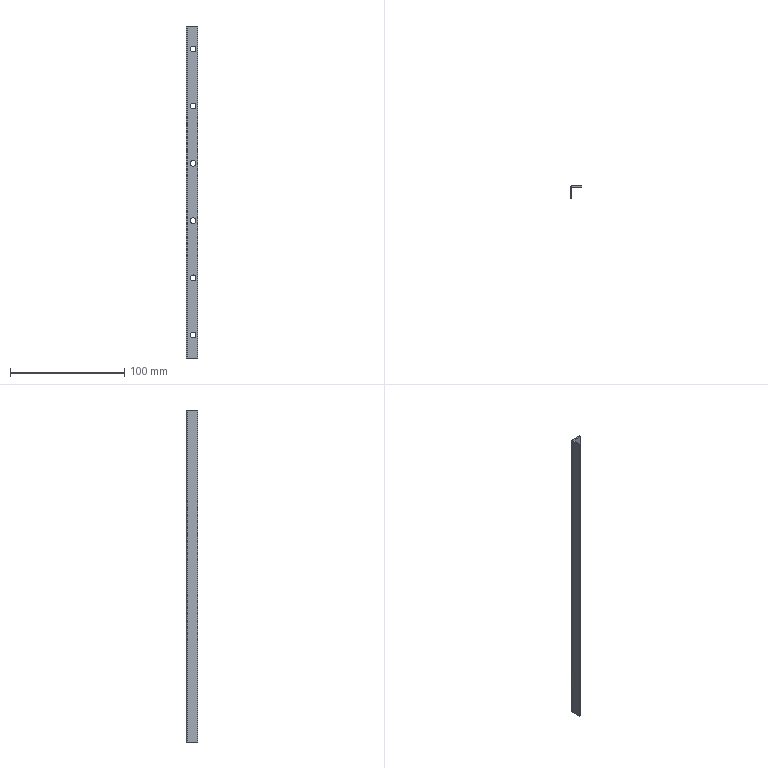Part | STEP file | RJWD-DY-0114_X2_75356C145B898_7 | 1 solid | 21 faces | box 10 x 10 x 290 mm | volume 5331 mm3 | cylinder 13 | plane 8 | commonest cylinder face diameters 5 x12 2.004 x1